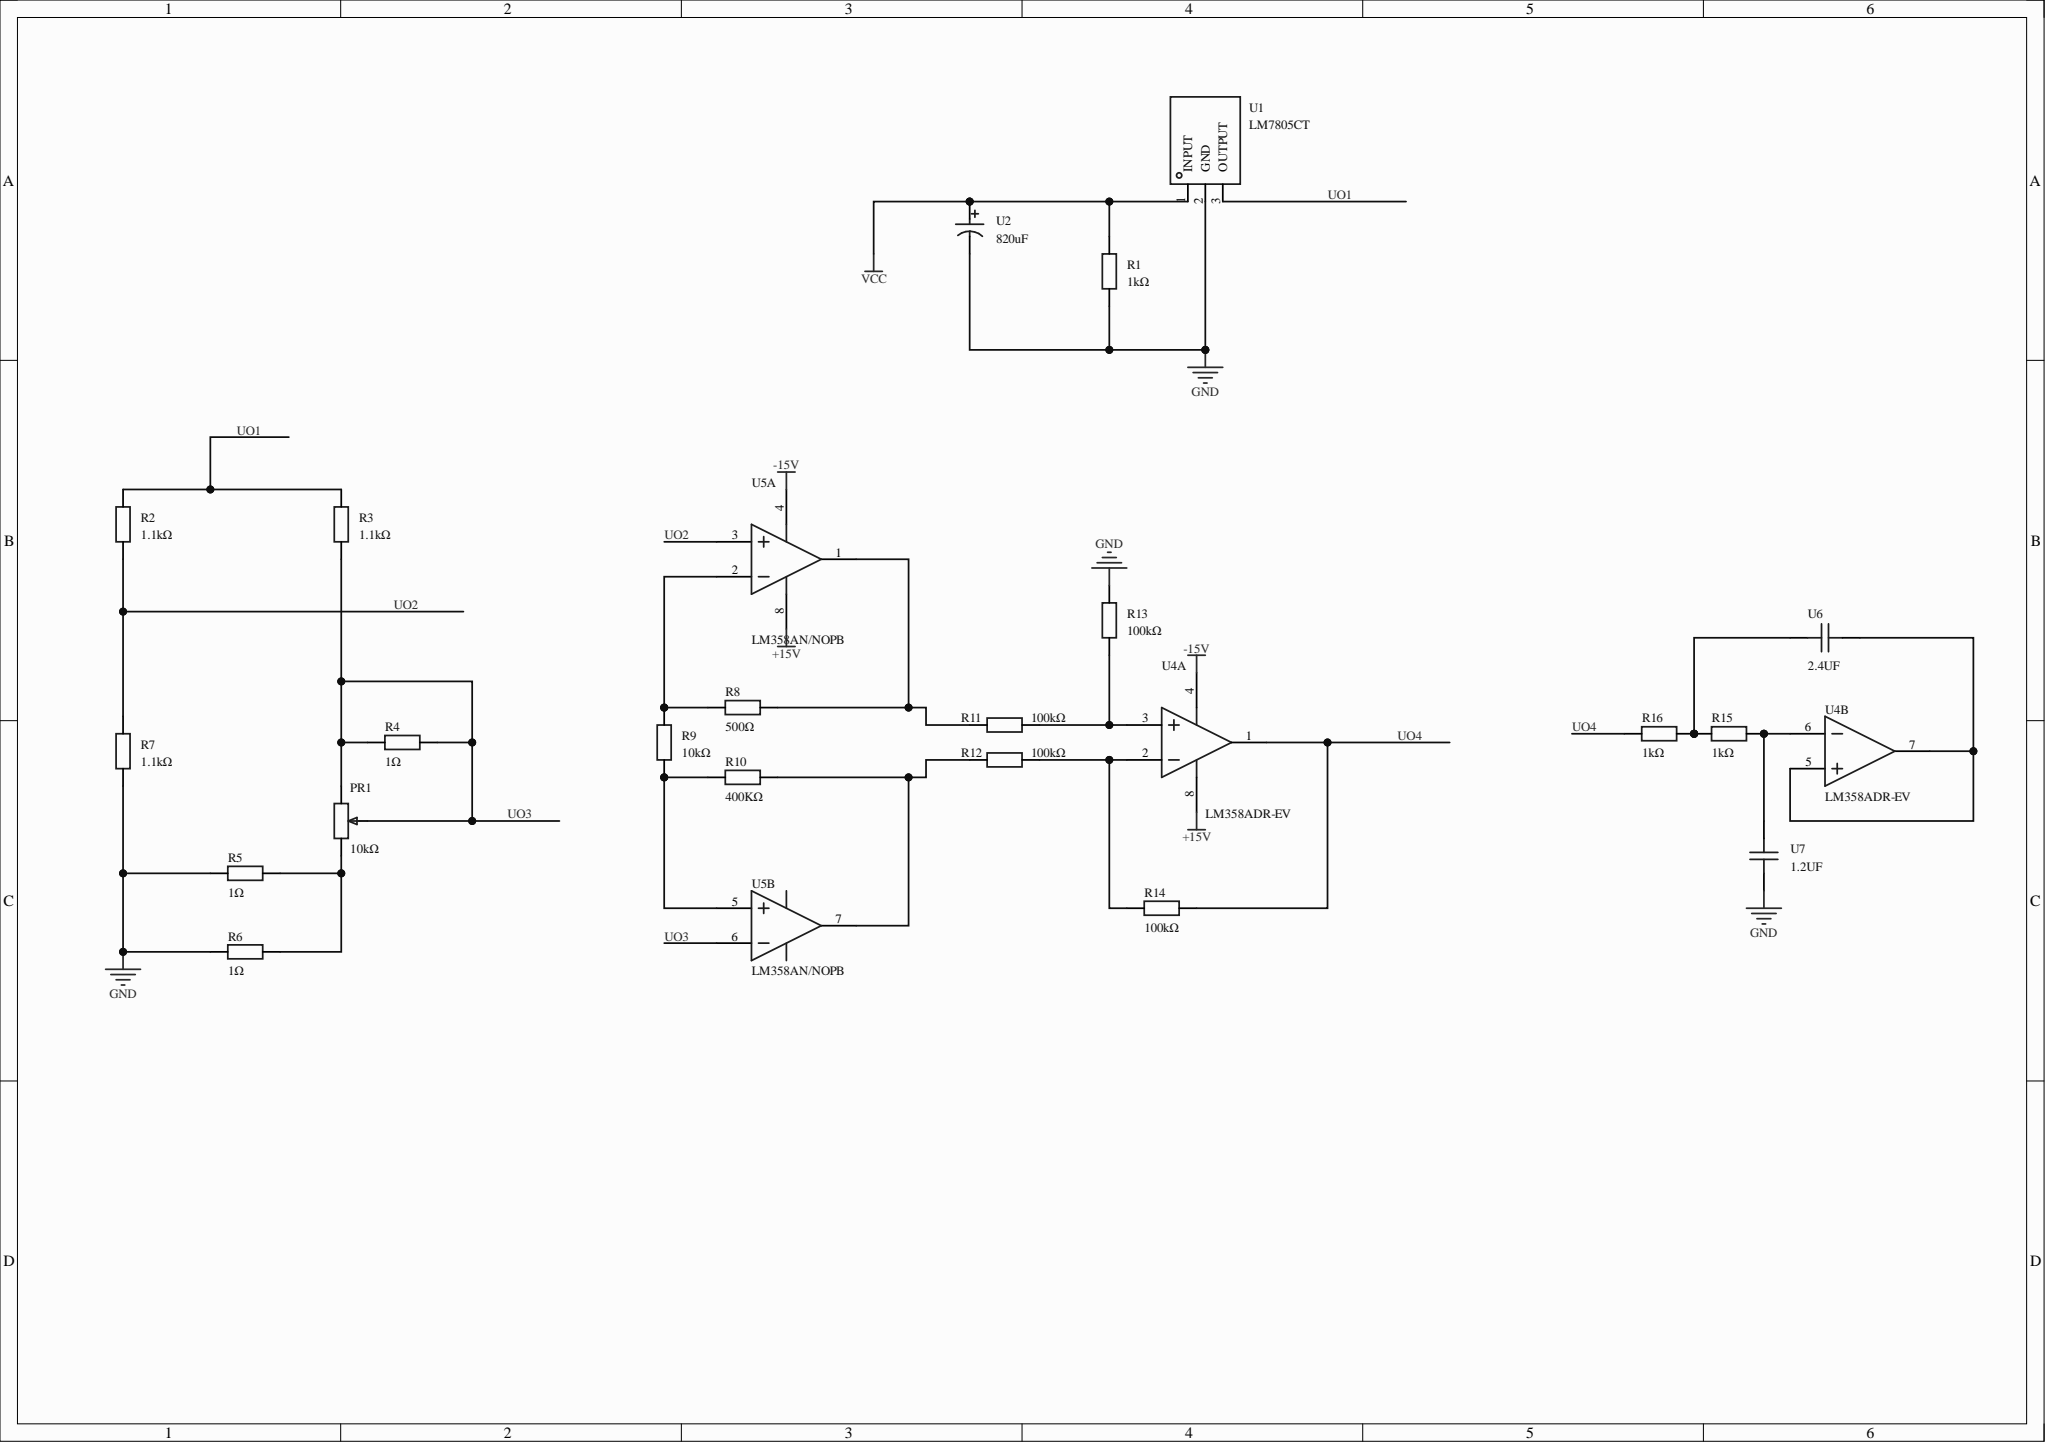Circuit board | Altium Designer | 23 parts | 18 nets
Bill of materials:
Comment,Description,Designator,Footprint,LibRef,Quantity
"10kΩ","","PR1","R_3296","R_3296","1"
"1kΩ","","R1, R15, R16","Res_1/8W","Res_AXIAL-1/8W","3"
"1.1kΩ","","R2, R3, R7","Res_1/8W","Res_AXIAL-1/8W","3"
"1Ω","","R4, R5, R6","Res_1/8W","Res_AXIAL-1/8W","3"
"500Ω","","R8","Res_1/8W","Res_AXIAL-1/8W","1"
"10kΩ","","R9","Res_1/8W","Res_AXIAL-1/8W","1"
"400KΩ","","R10","Res_1/8W","Res_AXIAL-1/8W","1"
"100kΩ","","R11, R12, R13, R14","Res_1/8W","Res_AXIAL-1/8W","4"
"LM7805CT","输出类型:固定;工作电压:35V;输出电压:5V;输出电流:1.5A;电源纹波抑制比(PSRR):62dB@(120Hz);输出极性:正极;","U1","TO-220-3_L10.0-W4.5-P2.54-L","LM7805CT","1"
"820uF","容值:820uF;精度:±20%;额定电压:200V;脚间距:10mm;等效串联电阻:-;纹波电流:1.75A@120Hz;","U2","CAP-TH_BD22.0-P10.00-D2.2-FD","LGG2D821MELZ40","1"
"LM358ADR-EV","放大器数:双路;输入失调电压(Vos):2mV;输入偏置电流(Ib):40nA;","U4","SOIC-8_L4.9-W3.9-P1.27-LS6.0-BL","LM358ADR-EV","1"
"LM358AN/NOPB","放大器数:2;轨到轨:-;增益带宽积(GBW):1MHz;输入失调电压(Vos):2mV;压摆率(SR):-;输入偏置电流(Ib):50nA;","U5","PDIP-8_L10.2-W6.5-P2.54-LS7.6-BL","LM358AN/NOPB","1"
"2.4UF","","U6","CAP-TH_L5.0-W2.5-P5.00-D1.0","100nF","1"
"1.2UF","","U7","CAP-TH_L5.0-W2.5-P5.00-D1.0","100nF","1"
Netlist (Protel format):
[
PR1
R_3296
10kΩ



]
[
R1
Res_1/8W
1kΩ



]
[
R2
Res_1/8W
1.1kΩ



]
[
R3
Res_1/8W
1.1kΩ



]
[
R4
Res_1/8W
1Ω



]
[
R5
Res_1/8W
1Ω



]
[
R6
Res_1/8W
1Ω



]
[
R7
Res_1/8W
1.1kΩ



]
[
R8
Res_1/8W
500Ω



]
[
R9
Res_1/8W
10kΩ



]
[
R10
Res_1/8W
400KΩ



]
[
R11
Res_1/8W
100kΩ



]
[
R12
Res_1/8W
100kΩ



]
[
R13
Res_1/8W
100kΩ



]
[
R14
Res_1/8W
100kΩ



]
[
R15
Res_1/8W
1kΩ



]
[
R16
Res_1/8W
1kΩ



]
[
U1
TO-220-3_L10.0-W4.5-P2.54-L
LM7805CT



]
[
U2
CAP-TH_BD22.0-P10.00-D2.2-FD
820uF



]
[
U4
SOIC-8_L4.9-W3.9-P1.27-LS6.0-BL
LM358ADR-EV



]
[
U5
PDIP-8_L10.2-W6.5-P2.54-LS7.6-BL
LM358AN/NOPB



]
[
U6
CAP-TH_L5.0-W2.5-P5.00-D1.0
2.4UF



]
[
U7
CAP-TH_L5.0-W2.5-P5.00-D1.0
1.2UF



]
(
VCC
R1-2
U1-1
U2-1
)
(
UO4
R14-1
R16-1
U4-1
)
(
UO3
PR1-2
PR1-3
R3-1
R4-1
R4-2
U5-6
)
(
UO2
R2-1
R7-2
U5-3
)
(
UO1
R2-2
R3-2
U1-3
)
(
NetU4_5
U4-5
U4-7
U6-1
)
(
NetR15_2
R15-2
U4-6
U7-1
)
(
NetR15_1
R15-1
R16-2
U6-2
)
(
NetR12_2
R12-2
R14-2
U4-2
)
(
NetR11_2
R11-2
R13-1
U4-3
)
(
NetR10_2
R10-2
R12-1
U5-7
)
(
NetR9_1
R9-1
R10-1
U5-5
)
(
NetR8_2
R8-2
R11-1
U5-1
)
(
NetR8_1
R8-1
R9-2
U5-2
)
(
NetPR1_1
PR1-1
R5-1
R6-1
)
(
GND
R1-1
R5-2
R6-2
R7-1
R13-2
U1-2
U2-2
U7-2
)
(
-15V
U4-4
U5-4
)
(
+15V
U4-8
U5-8
)